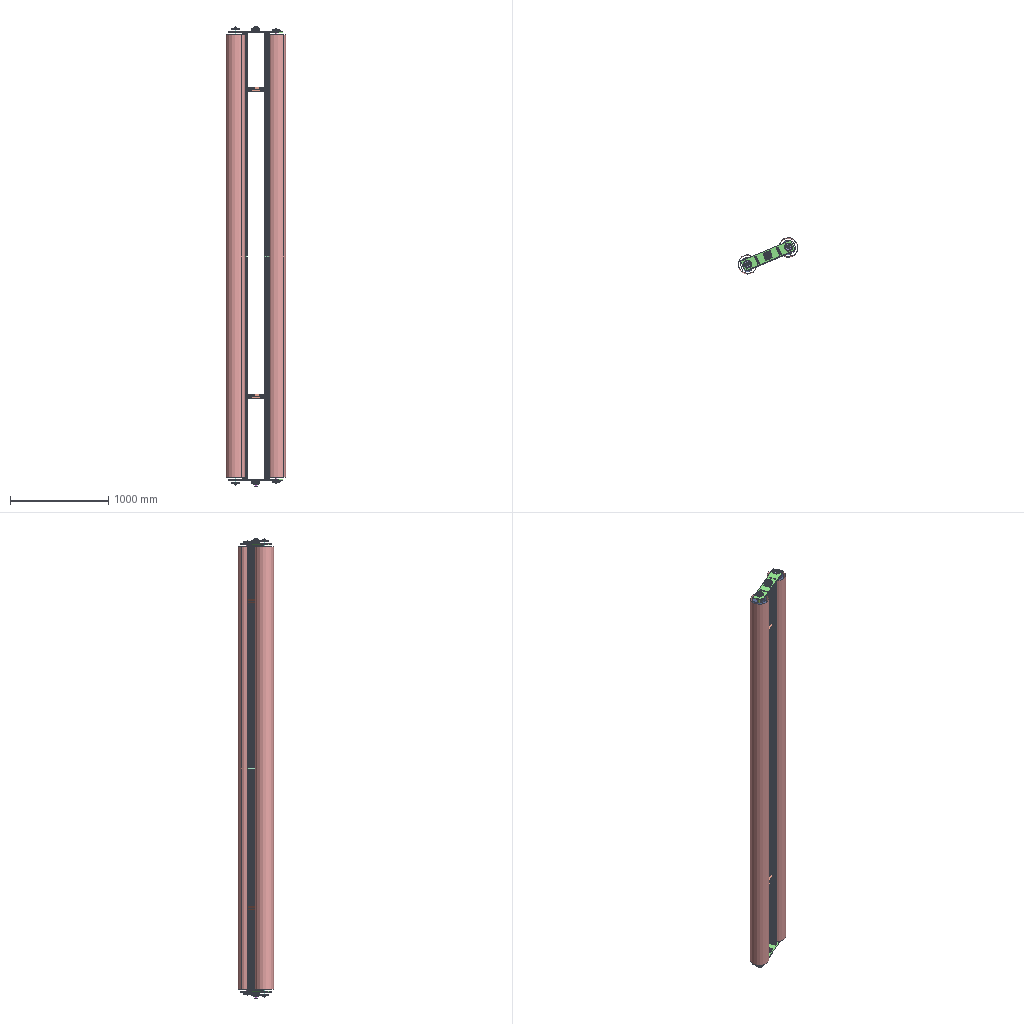Assembly | SolidWorks | 26 different items | 39 placed | box 604 x 361 x 4680 mm
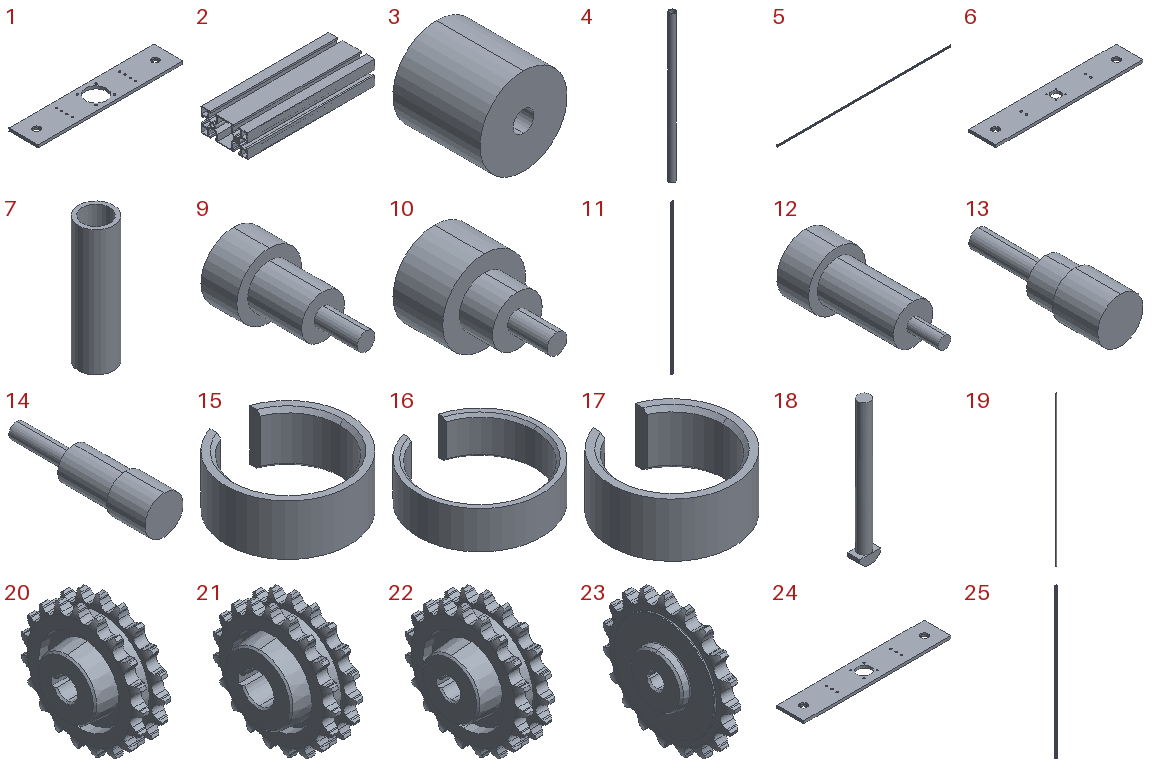Parts list (item | name | quantity | size | volume | features):
1 | - | x2 | 550 x 110 x 10 mm | 540695 mm3 | features ICE 5, Extrusion 1, Fillet 1, HoleWzd 1, MirrorPattern 1
2 | - | x2 | 220 x 80 x 40 mm | 163035 mm3 | features WeldMemberFeat 1, WeldmentFeature 1
3 | - | x1 | 25 x 25 x 25 mm | 11565 mm3 | features Extrusion 1
4 | - | x2 | 190 x 190 x 4500 mm | 116967 mm3 | features Extrusion 1, ICE 1
5 | - | x1 | 4546 x 20 x 40 mm | 1364953 mm3 | features HoleWzd 1, WeldMemberFeat 1, WeldmentFeature 1
6 | - | x1 | 550 x 100 x 10 mm | 528570 mm3 | features ICE 5, Extrusion 1, Fillet 1, HoleWzd 1, MirrorPattern 1
7 | - | x1 | 9 x 9 x 32 mm | 804.248 mm3 | features Extrusion 1
8 | - | x1 | - | - | features Boss 3, CurvePattern 2, Chamfer 1, CompositeCurve 1, Extrusion 1, MirrorPattern 1, MirrorSolid 1
9 | - | x1 | 18 x 37 x 18 mm | 4200 mm3 | features ICE 3, Extrusion 1
10 | - | x2 | 25 x 37 x 25 mm | 7911 mm3 | features ICE 3, Extrusion 1
11 | - | x2 | 80 x 20 x 4546 mm | 2507089 mm3 | features MBimport 1, MoveFace 1
12 | - | x1 | 18 x 44 x 18 mm | 5338 mm3 | features ICE 3, Extrusion 1
13 | - | x2 | 20 x 62.8 x 20 mm | 10660 mm3 | features ICE 3, Extrusion 1
14 | - | x2 | 20 x 77.2 x 20 mm | 13929 mm3 | features ICE 3, Extrusion 1
15 | - | x1 | 17 x 16.543 x 7 mm | 415.187 mm3 | features Chamfer 1, Extrusion 1, ICE 1
16 | - | x2 | 23 x 22.531 x 7 mm | 585.831 mm3 | features Chamfer 1, Extrusion 1, ICE 1
17 | - | x1 | 16 x 15.512 x 7 mm | 385.007 mm3 | features Chamfer 1, Extrusion 1, ICE 1
18 | - | x1 | 10 x 6 x 69.5 mm | 2064 mm3 | features Extrusion 1, ICE 1
19 | - | x2 | 35 x 35 x 4500 mm | 1357168 mm3 | features Extrusion 1
20 | - | x1 | 40 x 81.595 x 81.862 mm | 93771 mm3 | features Cut 2, Revolution 2, Chamfer 1, CirPattern 1, LPattern 1
21 | - | x2 | 40 x 81.595 x 81.862 mm | 99191 mm3 | features Cut 2, Revolution 2, Chamfer 1, CirPattern 1, LPattern 1
22 | - | x1 | 40 x 81.595 x 81.862 mm | 92773 mm3 | features Cut 2, Revolution 2, Chamfer 1, CirPattern 1, LPattern 1
23 | - | x4 | 20 x 81.595 x 81.862 mm | 45176 mm3 | features Cut 2, Revolution 2, Chamfer 1, CirPattern 1, Fillet 1, MirrorPattern 1
24 | - | x1 | 550 x 100 x 10 mm | 517578 mm3 | features ICE 5, Extrusion 1, Fillet 1, HoleWzd 1, MirrorPattern 1
25 | - | x1 | 60 x 20 x 4546 mm | 1925976 mm3 | features MBimport 1, MoveFace 1
26 | deep groove ball bearings gb | x1 | - | - | -
Mates (type | each side: item.copy, entity, surface, feature):
Concentric | 13.1 face cylinder Boss-Extrude3 | 23.1 face cylinder Revolve1
Coincident | 13.1 face plane Boss-Extrude2 | 23.1 face plane Revolve2
Concentric | 14.1 face cylinder Boss-Extrude3 | 23.2 face cylinder Revolve1
Coincident | 14.1 face plane Boss-Extrude2 | 23.2 face plane Revolve2
Concentric | 13.2 face cylinder Boss-Extrude3 | 23.3 face cylinder Revolve1
Coincident | 13.2 face plane Boss-Extrude2 | 23.3 face plane Revolve2
Concentric | 14.2 face cylinder Boss-Extrude3 | 23.4 face cylinder Revolve1
Coincident | 14.2 face plane Boss-Extrude2 | 23.4 face plane Revolve2
Coincident | 14.2 face plane Cut-Extrude1 | 23.4 face plane Cut-Extrude2
Coincident | 13.2 face plane Cut-Extrude1 | 23.3 face plane Cut-Extrude2
Coincident | 14.1 face plane Cut-Extrude1 | 23.2 face plane Cut-Extrude2
Coincident | 13.1 face plane Cut-Extrude1 | 23.1 face plane Cut-Extrude2
Concentric | 4.1 face cylinder Boss-Extrude2 | 19.1 face cylinder Boss-Extrude1
Concentric | 4.2 face cylinder Boss-Extrude2 | 19.2 face cylinder Boss-Extrude1
Coincident | 21.1 face plane Revolve2 | 16.1 face plane Boss-Extrude1
Coincident | 16.2 face plane Boss-Extrude1 | 21.2 face plane Revolve2
Concentric | 21.1 face cylinder Revolve2 | 10.1 face cylinder Boss-Extrude2
Coincident | 21.1 face plane Revolve2 | 10.1 face plane Boss-Extrude3
Concentric | 21.2 face cylinder Revolve2 | 10.2 face cylinder Boss-Extrude2
Coincident | 21.2 face plane Revolve2 | 10.2 face plane Boss-Extrude3
Coincident | 1.1 face plane Boss-Extrude1 | 11.1 face plane 2080 Profile.step
Concentric | 1.1 face cylinder Cut-Extrude6 | 11.1 face cylinder 2080 Profile.step | 2 times
Coincident | 1.1 face plane Boss-Extrude1 | 11.2 face plane 2080 Profile.step
Concentric | 1.1 face cylinder Cut-Extrude6 | 11.2 face cylinder 2080 Profile.step | 2 times
Coincident | 11.2 face plane 2080 Profile.step | 2.1 face plane Aluminum profile 40 X 80L X R0.3(1) | 2 times
Coincident | 11.2 face plane 2080 Profile.step | 2.2 face plane Aluminum profile 40 X 80L X R0.3(1) | 2 times